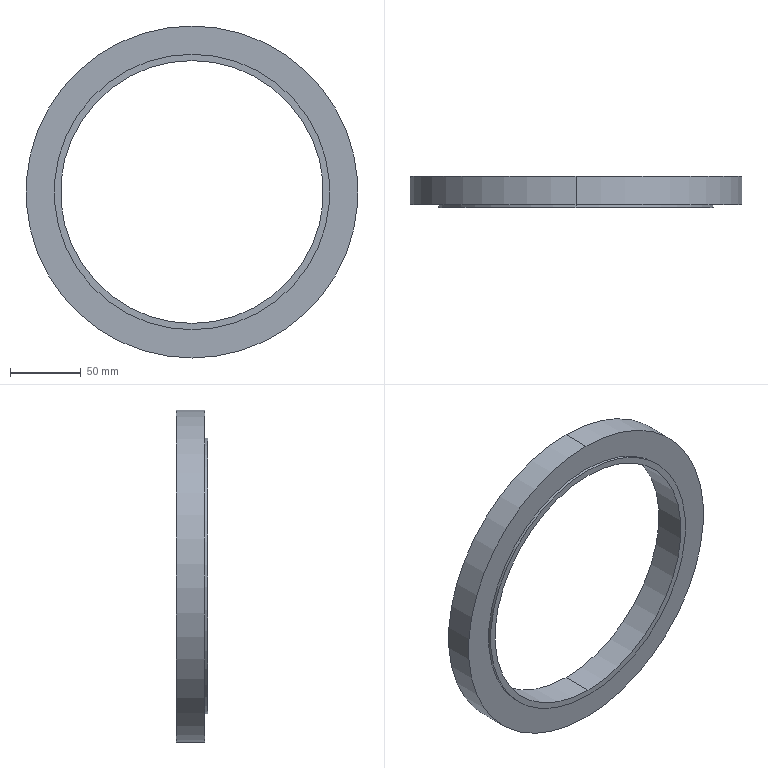Part | SolidWorks | features CirPattern 1, FlatPattern 1, HoleWzd 1, ICE 1, SMBaseFlange 1, SheetMetal 1 | 1 solid | 33 faces | box 235 x 22 x 235 mm | volume 321081 mm3 | cylinder 18 | cone 12 | plane 3 | commonest cylinder face diameters 10.2 x12 186 x2 195 x2 235 x2
STEP:
#1=CARTESIAN_POINT('',(90.933,-16.,-57.6));
#2=VERTEX_POINT('',#1);
#3=CARTESIAN_POINT('',(90.933,-16.,-47.4));
#4=VERTEX_POINT('',#3);
#5=CARTESIAN_POINT('',(90.933,-16.,-52.5));
#6=DIRECTION('',(0.,1.,0.));
#7=DIRECTION('',(0.,0.,1.));
#8=AXIS2_PLACEMENT_3D('',#5,#6,#7);
#9=CIRCLE('',#8,5.1);
#10=EDGE_CURVE('',#2,#4,#9,.T.);
#11=ORIENTED_EDGE('',*,*,#10,.F.);
#12=CARTESIAN_POINT('',(90.933,0.,-57.6));
#13=VERTEX_POINT('',#12);
#14=CARTESIAN_POINT('',(90.933,0.,-57.6));
#15=DIRECTION('',(0.,1.,0.));
#16=VECTOR('',#15,1000.);
#17=LINE('',#14,#16);
#18=EDGE_CURVE('',#2,#13,#17,.T.);
#19=ORIENTED_EDGE('',*,*,#18,.T.);
#20=CARTESIAN_POINT('',(90.933,0.,-47.4));
#21=VERTEX_POINT('',#20);
#22=CARTESIAN_POINT('',(90.933,0.,-52.5));
#23=DIRECTION('',(0.,1.,0.));
#24=DIRECTION('',(0.,0.,1.));
#25=AXIS2_PLACEMENT_3D('',#22,#23,#24);
#26=CIRCLE('',#25,5.1);
#27=EDGE_CURVE('',#13,#21,#26,.T.);
#28=ORIENTED_EDGE('',*,*,#27,.T.);
#29=CARTESIAN_POINT('',(90.933,0.,-47.4));
#30=DIRECTION('',(0.,1.,0.));
#31=VECTOR('',#30,1000.);
#32=LINE('',#29,#31);
#33=EDGE_CURVE('',#4,#21,#32,.T.);
#34=ORIENTED_EDGE('',*,*,#33,.F.);
#35=EDGE_LOOP('',(#11,#19,#28,#34));
#36=FACE_OUTER_BOUND('',#35,.T.);
#37=CARTESIAN_POINT('',(90.933,0.,-52.5));
#38=DIRECTION('',(0.,1.,0.));
#39=DIRECTION('',(0.,0.,1.));
#40=AXIS2_PLACEMENT_3D('',#37,#38,#39);
#41=CYLINDRICAL_SURFACE('',#40,5.1);
#42=ADVANCED_FACE('',(#36),#41,.F.);
#43=CARTESIAN_POINT('',(90.933,-19.064,-52.5));
#44=VERTEX_POINT('',#43);
#45=CARTESIAN_POINT('',(90.933,-16.,-47.4));
#46=DIRECTION('',(0.,0.515,0.8572));
#47=VECTOR('',#46,1000.);
#48=LINE('',#45,#47);
#49=EDGE_CURVE('',#44,#4,#48,.T.);
#50=ORIENTED_EDGE('',*,*,#49,.F.);
#51=CARTESIAN_POINT('',(90.933,-16.,-57.6));
#52=DIRECTION('',(0.,0.515,-0.8572));
#53=VECTOR('',#52,1000.);
#54=LINE('',#51,#53);
#55=EDGE_CURVE('',#44,#2,#54,.T.);
#56=ORIENTED_EDGE('',*,*,#55,.T.);
#57=ORIENTED_EDGE('',*,*,#10,.T.);
#58=EDGE_LOOP('',(#50,#56,#57));
#59=FACE_OUTER_BOUND('',#58,.T.);
#60=CARTESIAN_POINT('',(90.933,-16.,-52.5));
#61=DIRECTION('',(0.,1.,0.));
#62=DIRECTION('',(0.,0.,1.));
#63=AXIS2_PLACEMENT_3D('',#60,#61,#62);
#64=CONICAL_SURFACE('',#63,5.1,1.03);
#65=ADVANCED_FACE('',(#59),#64,.F.);
#66=CARTESIAN_POINT('',(90.933,-16.,47.4));
#67=VERTEX_POINT('',#66);
#68=CARTESIAN_POINT('',(90.933,-16.,57.6));
#69=VERTEX_POINT('',#68);
#70=CARTESIAN_POINT('',(90.933,-16.,52.5));
#71=DIRECTION('',(0.,1.,0.));
#72=DIRECTION('',(0.,0.,1.));
#73=AXIS2_PLACEMENT_3D('',#70,#71,#72);
#74=CIRCLE('',#73,5.1);
#75=EDGE_CURVE('',#67,#69,#74,.T.);
#76=ORIENTED_EDGE('',*,*,#75,.F.);
#77=CARTESIAN_POINT('',(90.933,0.,47.4));
#78=VERTEX_POINT('',#77);
#79=CARTESIAN_POINT('',(90.933,0.,47.4));
#80=DIRECTION('',(0.,1.,0.));
#81=VECTOR('',#80,1000.);
#82=LINE('',#79,#81);
#83=EDGE_CURVE('',#67,#78,#82,.T.);
#84=ORIENTED_EDGE('',*,*,#83,.T.);
#85=CARTESIAN_POINT('',(90.933,0.,57.6));
#86=VERTEX_POINT('',#85);
#87=CARTESIAN_POINT('',(90.933,0.,52.5));
#88=DIRECTION('',(0.,1.,0.));
#89=DIRECTION('',(0.,0.,1.));
#90=AXIS2_PLACEMENT_3D('',#87,#88,#89);
#91=CIRCLE('',#90,5.1);
#92=EDGE_CURVE('',#78,#86,#91,.T.);
#93=ORIENTED_EDGE('',*,*,#92,.T.);
#94=CARTESIAN_POINT('',(90.933,0.,57.6));
#95=DIRECTION('',(0.,1.,0.));
#96=VECTOR('',#95,1000.);
#97=LINE('',#94,#96);
#98=EDGE_CURVE('',#69,#86,#97,.T.);
#99=ORIENTED_EDGE('',*,*,#98,.F.);
#100=EDGE_LOOP('',(#76,#84,#93,#99));
#101=FACE_OUTER_BOUND('',#100,.T.);
#102=CARTESIAN_POINT('',(90.933,0.,52.5));
#103=DIRECTION('',(0.,1.,0.));
#104=DIRECTION('',(0.,0.,1.));
#105=AXIS2_PLACEMENT_3D('',#102,#103,#104);
#106=CYLINDRICAL_SURFACE('',#105,5.1);
#107=ADVANCED_FACE('',(#101),#106,.F.);
#108=CARTESIAN_POINT('',(90.933,-19.064,52.5));
#109=VERTEX_POINT('',#108);
#110=CARTESIAN_POINT('',(90.933,-16.,57.6));
#111=DIRECTION('',(0.,0.515,0.8572));
#112=VECTOR('',#111,1000.);
#113=LINE('',#110,#112);
#114=EDGE_CURVE('',#109,#69,#113,.T.);
#115=ORIENTED_EDGE('',*,*,#114,.F.);
#116=CARTESIAN_POINT('',(90.933,-16.,47.4));
#117=DIRECTION('',(0.,0.515,-0.8572));
#118=VECTOR('',#117,1000.);
#119=LINE('',#116,#118);
#120=EDGE_CURVE('',#109,#67,#119,.T.);
#121=ORIENTED_EDGE('',*,*,#120,.T.);
#122=ORIENTED_EDGE('',*,*,#75,.T.);
#123=EDGE_LOOP('',(#115,#121,#122));
#124=FACE_OUTER_BOUND('',#123,.T.);
#125=CARTESIAN_POINT('',(90.933,-16.,52.5));
#126=DIRECTION('',(0.,1.,0.));
#127=DIRECTION('',(0.,0.,1.));
#128=AXIS2_PLACEMENT_3D('',#125,#126,#127);
#129=CONICAL_SURFACE('',#128,5.1,1.03);
#130=ADVANCED_FACE('',(#124),#129,.F.);
#131=CARTESIAN_POINT('',(0.,-16.,99.9));
#132=VERTEX_POINT('',#131);
#133=CARTESIAN_POINT('',(0.,-16.,110.1));
#134=VERTEX_POINT('',#133);
#135=CARTESIAN_POINT('',(0.,-16.,105.));
#136=DIRECTION('',(0.,1.,0.));
#137=DIRECTION('',(0.,0.,1.));
#138=AXIS2_PLACEMENT_3D('',#135,#136,#137);
#139=CIRCLE('',#138,5.1);
#140=EDGE_CURVE('',#132,#134,#139,.T.);
#141=ORIENTED_EDGE('',*,*,#140,.F.);
#142=CARTESIAN_POINT('',(0.,0.,99.9));
#143=VERTEX_POINT('',#142);
#144=CARTESIAN_POINT('',(0.,0.,99.9));
#145=DIRECTION('',(0.,1.,0.));
#146=VECTOR('',#145,1000.);
#147=LINE('',#144,#146);
#148=EDGE_CURVE('',#132,#143,#147,.T.);
#149=ORIENTED_EDGE('',*,*,#148,.T.);
#150=CARTESIAN_POINT('',(0.,0.,110.1));
#151=VERTEX_POINT('',#150);
#152=CARTESIAN_POINT('',(0.,0.,105.));
#153=DIRECTION('',(0.,1.,0.));
#154=DIRECTION('',(0.,0.,1.));
#155=AXIS2_PLACEMENT_3D('',#152,#153,#154);
#156=CIRCLE('',#155,5.1);
#157=EDGE_CURVE('',#143,#151,#156,.T.);
#158=ORIENTED_EDGE('',*,*,#157,.T.);
#159=CARTESIAN_POINT('',(0.,0.,110.1));
#160=DIRECTION('',(0.,1.,0.));
#161=VECTOR('',#160,1000.);
#162=LINE('',#159,#161);
#163=EDGE_CURVE('',#134,#151,#162,.T.);
#164=ORIENTED_EDGE('',*,*,#163,.F.);
#165=EDGE_LOOP('',(#141,#149,#158,#164));
#166=FACE_OUTER_BOUND('',#165,.T.);
#167=CARTESIAN_POINT('',(0.,0.,105.));
#168=DIRECTION('',(0.,1.,0.));
#169=DIRECTION('',(0.,0.,1.));
#170=AXIS2_PLACEMENT_3D('',#167,#168,#169);
#171=CYLINDRICAL_SURFACE('',#170,5.1);
#172=ADVANCED_FACE('',(#166),#171,.F.);
#173=CARTESIAN_POINT('',(0.,-19.064,105.));
#174=VERTEX_POINT('',#173);
#175=CARTESIAN_POINT('',(0.,-16.,110.1));
#176=DIRECTION('',(0.,0.515,0.8572));
#177=VECTOR('',#176,1000.);
#178=LINE('',#175,#177);
#179=EDGE_CURVE('',#174,#134,#178,.T.);
#180=ORIENTED_EDGE('',*,*,#179,.F.);
#181=CARTESIAN_POINT('',(0.,-16.,99.9));
#182=DIRECTION('',(0.,0.515,-0.8572));
#183=VECTOR('',#182,1000.);
#184=LINE('',#181,#183);
#185=EDGE_CURVE('',#174,#132,#184,.T.);
#186=ORIENTED_EDGE('',*,*,#185,.T.);
#187=ORIENTED_EDGE('',*,*,#140,.T.);
#188=EDGE_LOOP('',(#180,#186,#187));
#189=FACE_OUTER_BOUND('',#188,.T.);
#190=CARTESIAN_POINT('',(0.,-16.,105.));
#191=DIRECTION('',(0.,1.,0.));
#192=DIRECTION('',(0.,0.,1.));
#193=AXIS2_PLACEMENT_3D('',#190,#191,#192);
#194=CONICAL_SURFACE('',#193,5.1,1.03);
#195=ADVANCED_FACE('',(#189),#194,.F.);
#196=CARTESIAN_POINT('',(-90.933,-16.,47.4));
#197=VERTEX_POINT('',#196);
#198=CARTESIAN_POINT('',(-90.933,-16.,57.6));
#199=VERTEX_POINT('',#198);
#200=CARTESIAN_POINT('',(-90.933,-16.,52.5));
#201=DIRECTION('',(0.,1.,0.));
#202=DIRECTION('',(0.,0.,1.));
#203=AXIS2_PLACEMENT_3D('',#200,#201,#202);
#204=CIRCLE('',#203,5.1);
#205=EDGE_CURVE('',#197,#199,#204,.T.);
#206=ORIENTED_EDGE('',*,*,#205,.F.);
#207=CARTESIAN_POINT('',(-90.933,0.,47.4));
#208=VERTEX_POINT('',#207);
#209=CARTESIAN_POINT('',(-90.933,0.,47.4));
#210=DIRECTION('',(0.,1.,0.));
#211=VECTOR('',#210,1000.);
#212=LINE('',#209,#211);
#213=EDGE_CURVE('',#197,#208,#212,.T.);
#214=ORIENTED_EDGE('',*,*,#213,.T.);
#215=CARTESIAN_POINT('',(-90.933,0.,57.6));
#216=VERTEX_POINT('',#215);
#217=CARTESIAN_POINT('',(-90.933,0.,52.5));
#218=DIRECTION('',(0.,1.,0.));
#219=DIRECTION('',(0.,0.,1.));
#220=AXIS2_PLACEMENT_3D('',#217,#218,#219);
#221=CIRCLE('',#220,5.1);
#222=EDGE_CURVE('',#208,#216,#221,.T.);
#223=ORIENTED_EDGE('',*,*,#222,.T.);
#224=CARTESIAN_POINT('',(-90.933,0.,57.6));
#225=DIRECTION('',(0.,1.,0.));
#226=VECTOR('',#225,1000.);
#227=LINE('',#224,#226);
#228=EDGE_CURVE('',#199,#216,#227,.T.);
#229=ORIENTED_EDGE('',*,*,#228,.F.);
#230=EDGE_LOOP('',(#206,#214,#223,#229));
#231=FACE_OUTER_BOUND('',#230,.T.);
#232=CARTESIAN_POINT('',(-90.933,0.,52.5));
#233=DIRECTION('',(0.,1.,0.));
#234=DIRECTION('',(0.,0.,1.));
#235=AXIS2_PLACEMENT_3D('',#232,#233,#234);
#236=CYLINDRICAL_SURFACE('',#235,5.1);
#237=ADVANCED_FACE('',(#231),#236,.F.);
#238=CARTESIAN_POINT('',(-90.933,-19.064,52.5));
#239=VERTEX_POINT('',#238);
#240=CARTESIAN_POINT('',(-90.933,-16.,57.6));
#241=DIRECTION('',(0.,0.515,0.8572));
#242=VECTOR('',#241,1000.);
#243=LINE('',#240,#242);
#244=EDGE_CURVE('',#239,#199,#243,.T.);
#245=ORIENTED_EDGE('',*,*,#244,.F.);
#246=CARTESIAN_POINT('',(-90.933,-16.,47.4));
#247=DIRECTION('',(0.,0.515,-0.8572));
#248=VECTOR('',#247,1000.);
#249=LINE('',#246,#248);
#250=EDGE_CURVE('',#239,#197,#249,.T.);
#251=ORIENTED_EDGE('',*,*,#250,.T.);
#252=ORIENTED_EDGE('',*,*,#205,.T.);
#253=EDGE_LOOP('',(#245,#251,#252));
#254=FACE_OUTER_BOUND('',#253,.T.);
#255=CARTESIAN_POINT('',(-90.933,-16.,52.5));
#256=DIRECTION('',(0.,1.,0.));
#257=DIRECTION('',(0.,0.,1.));
#258=AXIS2_PLACEMENT_3D('',#255,#256,#257);
#259=CONICAL_SURFACE('',#258,5.1,1.03);
#260=ADVANCED_FACE('',(#254),#259,.F.);
#261=CARTESIAN_POINT('',(-90.933,-16.,-57.6));
#262=VERTEX_POINT('',#261);
#263=CARTESIAN_POINT('',(-90.933,-16.,-47.4));
#264=VERTEX_POINT('',#263);
#265=CARTESIAN_POINT('',(-90.933,-16.,-52.5));
#266=DIRECTION('',(0.,1.,0.));
#267=DIRECTION('',(0.,0.,1.));
#268=AXIS2_PLACEMENT_3D('',#265,#266,#267);
#269=CIRCLE('',#268,5.1);
#270=EDGE_CURVE('',#262,#264,#269,.T.);
#271=ORIENTED_EDGE('',*,*,#270,.F.);
#272=CARTESIAN_POINT('',(-90.933,0.,-57.6));
#273=VERTEX_POINT('',#272);
#274=CARTESIAN_POINT('',(-90.933,0.,-57.6));
#275=DIRECTION('',(0.,1.,0.));
#276=VECTOR('',#275,1000.);
#277=LINE('',#274,#276);
#278=EDGE_CURVE('',#262,#273,#277,.T.);
#279=ORIENTED_EDGE('',*,*,#278,.T.);
#280=CARTESIAN_POINT('',(-90.933,0.,-47.4));
#281=VERTEX_POINT('',#280);
#282=CARTESIAN_POINT('',(-90.933,0.,-52.5));
#283=DIRECTION('',(0.,1.,0.));
#284=DIRECTION('',(0.,0.,1.));
#285=AXIS2_PLACEMENT_3D('',#282,#283,#284);
#286=CIRCLE('',#285,5.1);
#287=EDGE_CURVE('',#273,#281,#286,.T.);
#288=ORIENTED_EDGE('',*,*,#287,.T.);
#289=CARTESIAN_POINT('',(-90.933,0.,-47.4));
#290=DIRECTION('',(0.,1.,0.));
#291=VECTOR('',#290,1000.);
#292=LINE('',#289,#291);
#293=EDGE_CURVE('',#264,#281,#292,.T.);
#294=ORIENTED_EDGE('',*,*,#293,.F.);
#295=EDGE_LOOP('',(#271,#279,#288,#294));
#296=FACE_OUTER_BOUND('',#295,.T.);
#297=CARTESIAN_POINT('',(-90.933,0.,-52.5));
#298=DIRECTION('',(0.,1.,0.));
#299=DIRECTION('',(0.,0.,1.));
#300=AXIS2_PLACEMENT_3D('',#297,#298,#299);
#301=CYLINDRICAL_SURFACE('',#300,5.1);
#302=ADVANCED_FACE('',(#296),#301,.F.);
#303=CARTESIAN_POINT('',(-90.933,-19.064,-52.5));
#304=VERTEX_POINT('',#303);
#305=CARTESIAN_POINT('',(-90.933,-16.,-47.4));
#306=DIRECTION('',(0.,0.515,0.8572));
#307=VECTOR('',#306,1000.);
#308=LINE('',#305,#307);
#309=EDGE_CURVE('',#304,#264,#308,.T.);
#310=ORIENTED_EDGE('',*,*,#309,.F.);
#311=CARTESIAN_POINT('',(-90.933,-16.,-57.6));
#312=DIRECTION('',(0.,0.515,-0.8572));
#313=VECTOR('',#312,1000.);
#314=LINE('',#311,#313);
#315=EDGE_CURVE('',#304,#262,#314,.T.);
#316=ORIENTED_EDGE('',*,*,#315,.T.);
#317=ORIENTED_EDGE('',*,*,#270,.T.);
#318=EDGE_LOOP('',(#310,#316,#317));
#319=FACE_OUTER_BOUND('',#318,.T.);
#320=CARTESIAN_POINT('',(-90.933,-16.,-52.5));
#321=DIRECTION('',(0.,1.,0.));
#322=DIRECTION('',(0.,0.,1.));
#323=AXIS2_PLACEMENT_3D('',#320,#321,#322);
#324=CONICAL_SURFACE('',#323,5.1,1.03);
#325=ADVANCED_FACE('',(#319),#324,.F.);
#326=CARTESIAN_POINT('',(0.,-16.,-110.1));
#327=VERTEX_POINT('',#326);
#328=CARTESIAN_POINT('',(0.,-16.,-99.9));
#329=VERTEX_POINT('',#328);
#330=CARTESIAN_POINT('',(0.,-16.,-105.));
#331=DIRECTION('',(0.,1.,0.));
#332=DIRECTION('',(0.,0.,1.));
#333=AXIS2_PLACEMENT_3D('',#330,#331,#332);
#334=CIRCLE('',#333,5.1);
#335=EDGE_CURVE('',#327,#329,#334,.T.);
#336=ORIENTED_EDGE('',*,*,#335,.F.);
#337=CARTESIAN_POINT('',(0.,0.,-110.1));
#338=VERTEX_POINT('',#337);
#339=CARTESIAN_POINT('',(0.,0.,-110.1));
#340=DIRECTION('',(0.,1.,0.));
#341=VECTOR('',#340,1000.);
#342=LINE('',#339,#341);
#343=EDGE_CURVE('',#327,#338,#342,.T.);
#344=ORIENTED_EDGE('',*,*,#343,.T.);
#345=CARTESIAN_POINT('',(0.,0.,-99.9));
#346=VERTEX_POINT('',#345);
#347=CARTESIAN_POINT('',(0.,0.,-105.));
#348=DIRECTION('',(0.,1.,0.));
#349=DIRECTION('',(0.,0.,1.));
#350=AXIS2_PLACEMENT_3D('',#347,#348,#349);
#351=CIRCLE('',#350,5.1);
#352=EDGE_CURVE('',#338,#346,#351,.T.);
#353=ORIENTED_EDGE('',*,*,#352,.T.);
#354=CARTESIAN_POINT('',(0.,0.,-99.9));
#355=DIRECTION('',(0.,1.,0.));
#356=VECTOR('',#355,1000.);
#357=LINE('',#354,#356);
#358=EDGE_CURVE('',#329,#346,#357,.T.);
#359=ORIENTED_EDGE('',*,*,#358,.F.);
#360=EDGE_LOOP('',(#336,#344,#353,#359));
#361=FACE_OUTER_BOUND('',#360,.T.);
#362=CARTESIAN_POINT('',(0.,0.,-105.));
#363=DIRECTION('',(0.,1.,0.));
#364=DIRECTION('',(0.,0.,1.));
#365=AXIS2_PLACEMENT_3D('',#362,#363,#364);
#366=CYLINDRICAL_SURFACE('',#365,5.1);
#367=ADVANCED_FACE('',(#361),#366,.F.);
#368=CARTESIAN_POINT('',(0.,-19.064,-105.));
#369=VERTEX_POINT('',#368);
#370=CARTESIAN_POINT('',(0.,-16.,-99.9));
#371=DIRECTION('',(0.,0.515,0.8572));
#372=VECTOR('',#371,1000.);
#373=LINE('',#370,#372);
#374=EDGE_CURVE('',#369,#329,#373,.T.);
#375=ORIENTED_EDGE('',*,*,#374,.F.);
#376=CARTESIAN_POINT('',(0.,-16.,-110.1));
#377=DIRECTION('',(0.,0.515,-0.8572));
#378=VECTOR('',#377,1000.);
#379=LINE('',#376,#378);
#380=EDGE_CURVE('',#369,#327,#379,.T.);
#381=ORIENTED_EDGE('',*,*,#380,.T.);
#382=ORIENTED_EDGE('',*,*,#335,.T.);
#383=EDGE_LOOP('',(#375,#381,#382));
#384=FACE_OUTER_BOUND('',#383,.T.);
#385=CARTESIAN_POINT('',(0.,-16.,-105.));
#386=DIRECTION('',(0.,1.,0.));
#387=DIRECTION('',(0.,0.,1.));
#388=AXIS2_PLACEMENT_3D('',#385,#386,#387);
#389=CONICAL_SURFACE('',#388,5.1,1.03);
#390=ADVANCED_FACE('',(#384),#389,.F.);
#391=CARTESIAN_POINT('',(0.,-20.,-97.5));
#392=VERTEX_POINT('',#391);
#393=CARTESIAN_POINT('',(0.,-20.,97.5));
#394=VERTEX_POINT('',#393);
#395=CARTESIAN_POINT('',(0.,-20.,0.));
#396=DIRECTION('',(0.,-1.,0.));
#397=DIRECTION('',(0.,0.,-1.));
#398=AXIS2_PLACEMENT_3D('',#395,#396,#397);
#399=CIRCLE('',#398,97.5);
#400=EDGE_CURVE('',#392,#394,#399,.T.);
#401=ORIENTED_EDGE('',*,*,#400,.T.);
#402=CARTESIAN_POINT('',(0.,-22.,97.5));
#403=VERTEX_POINT('',#402);
#404=CARTESIAN_POINT('',(0.,-20.,97.5));
#405=DIRECTION('',(0.,-1.,0.));
#406=VECTOR('',#405,1000.);
#407=LINE('',#404,#406);
#408=EDGE_CURVE('',#394,#403,#407,.T.);
#409=ORIENTED_EDGE('',*,*,#408,.T.);
#410=CARTESIAN_POINT('',(0.,-22.,-97.5));
#411=VERTEX_POINT('',#410);
#412=CARTESIAN_POINT('',(0.,-22.,0.));
#413=DIRECTION('',(0.,-1.,0.));
#414=DIRECTION('',(0.,0.,-1.));
#415=AXIS2_PLACEMENT_3D('',#412,#413,#414);
#416=CIRCLE('',#415,97.5);
#417=EDGE_CURVE('',#411,#403,#416,.T.);
#418=ORIENTED_EDGE('',*,*,#417,.F.);
#419=CARTESIAN_POINT('',(0.,-20.,-97.5));
#420=DIRECTION('',(0.,-1.,0.));
#421=VECTOR('',#420,1000.);
#422=LINE('',#419,#421);
#423=EDGE_CURVE('',#392,#411,#422,.T.);
#424=ORIENTED_EDGE('',*,*,#423,.F.);
#425=EDGE_LOOP('',(#401,#409,#418,#424));
#426=FACE_OUTER_BOUND('',#425,.T.);
#427=CARTESIAN_POINT('',(0.,-20.,0.));
#428=DIRECTION('',(0.,-1.,0.));
#429=DIRECTION('',(0.,0.,-1.));
#430=AXIS2_PLACEMENT_3D('',#427,#428,#429);
#431=CYLINDRICAL_SURFACE('',#430,97.5);
#432=ADVANCED_FACE('',(#426),#431,.T.);
#433=CARTESIAN_POINT('',(0.,-22.,-93.));
#434=VERTEX_POINT('',#433);
#435=CARTESIAN_POINT('',(0.,-22.,93.));
#436=VERTEX_POINT('',#435);
#437=CARTESIAN_POINT('',(0.,-22.,0.));
#438=DIRECTION('',(0.,1.,0.));
#439=DIRECTION('',(0.,0.,1.));
#440=AXIS2_PLACEMENT_3D('',#437,#438,#439);
#441=CIRCLE('',#440,93.);
#442=EDGE_CURVE('',#434,#436,#441,.T.);
#443=ORIENTED_EDGE('',*,*,#442,.F.);
#444=CARTESIAN_POINT('',(0.,0.,-93.));
#445=VERTEX_POINT('',#444);
#446=CARTESIAN_POINT('',(0.,-22.,-93.));
#447=DIRECTION('',(0.,1.,0.));
#448=VECTOR('',#447,1000.);
#449=LINE('',#446,#448);
#450=EDGE_CURVE('',#434,#445,#449,.T.);
#451=ORIENTED_EDGE('',*,*,#450,.T.);
#452=CARTESIAN_POINT('',(0.,0.,93.));
#453=VERTEX_POINT('',#452);
#454=CARTESIAN_POINT('',(0.,0.,0.));
#455=DIRECTION('',(0.,1.,0.));
#456=DIRECTION('',(0.,0.,1.));
#457=AXIS2_PLACEMENT_3D('',#454,#455,#456);
#458=CIRCLE('',#457,93.);
#459=EDGE_CURVE('',#445,#453,#458,.T.);
#460=ORIENTED_EDGE('',*,*,#459,.T.);
#461=CARTESIAN_POINT('',(0.,-22.,93.));
#462=DIRECTION('',(0.,1.,0.));
#463=VECTOR('',#462,1000.);
#464=LINE('',#461,#463);
#465=EDGE_CURVE('',#436,#453,#464,.T.);
#466=ORIENTED_EDGE('',*,*,#465,.F.);
#467=EDGE_LOOP('',(#443,#451,#460,#466));
#468=FACE_OUTER_BOUND('',#467,.T.);
#469=CARTESIAN_POINT('',(0.,-22.,0.));
#470=DIRECTION('',(0.,1.,0.));
#471=DIRECTION('',(0.,0.,1.));
#472=AXIS2_PLACEMENT_3D('',#469,#470,#471);
#473=CYLINDRICAL_SURFACE('',#472,93.);
#474=ADVANCED_FACE('',(#468),#473,.F.);
#475=CARTESIAN_POINT('',(0.,-20.,117.5));
#476=VERTEX_POINT('',#475);
#477=CARTESIAN_POINT('',(0.,-20.,-117.5));
#478=VERTEX_POINT('',#477);
#479=CARTESIAN_POINT('',(0.,-20.,0.));
#480=DIRECTION('',(0.,1.,0.));
#481=DIRECTION('',(0.,0.,-1.));
#482=AXIS2_PLACEMENT_3D('',#479,#480,#481);
#483=CIRCLE('',#482,117.5);
#484=EDGE_CURVE('',#476,#478,#483,.T.);
#485=ORIENTED_EDGE('',*,*,#484,.T.);
#486=CARTESIAN_POINT('',(0.,0.,-117.5));
#487=VERTEX_POINT('',#486);
#488=CARTESIAN_POINT('',(0.,-22.,-117.5));
#489=DIRECTION('',(0.,1.,0.));
#490=VECTOR('',#489,1000.);
#491=LINE('',#488,#490);
#492=EDGE_CURVE('',#478,#487,#491,.T.);
#493=ORIENTED_EDGE('',*,*,#492,.T.);
#494=CARTESIAN_POINT('',(0.,0.,117.5));
#495=VERTEX_POINT('',#494);
#496=CARTESIAN_POINT('',(0.,0.,0.));
#497=DIRECTION('',(0.,1.,0.));
#498=DIRECTION('',(0.,0.,1.));
#499=AXIS2_PLACEMENT_3D('',#496,#497,#498);
#500=CIRCLE('',#499,117.5);
#501=EDGE_CURVE('',#495,#487,#500,.T.);
#502=ORIENTED_EDGE('',*,*,#501,.F.);
#503=CARTESIAN_POINT('',(0.,-22.,117.5));
#504=DIRECTION('',(0.,1.,0.));
#505=VECTOR('',#504,1000.);
#506=LINE('',#503,#505);
#507=EDGE_CURVE('',#476,#495,#506,.T.);
#508=ORIENTED_EDGE('',*,*,#507,.F.);
#509=EDGE_LOOP('',(#485,#493,#502,#508));
#510=FACE_OUTER_BOUND('',#509,.T.);
#511=CARTESIAN_POINT('',(0.,-22.,0.));
#512=DIRECTION('',(0.,1.,0.));
#513=DIRECTION('',(0.,0.,1.));
#514=AXIS2_PLACEMENT_3D('',#511,#512,#513);
#515=CYLINDRICAL_SURFACE('',#514,117.5);
#516=ADVANCED_FACE('',(#510),#515,.T.);
#517=ORIENTED_EDGE('',*,*,#492,.F.);
#518=CARTESIAN_POINT('',(0.,-20.,0.));
#519=DIRECTION('',(0.,1.,0.));
#520=DIRECTION('',(0.,0.,-1.));
#521=AXIS2_PLACEMENT_3D('',#518,#519,#520);
#522=CIRCLE('',#521,117.5);
#523=EDGE_CURVE('',#478,#476,#522,.T.);
#524=ORIENTED_EDGE('',*,*,#523,.T.);
#525=ORIENTED_EDGE('',*,*,#507,.T.);
#526=CARTESIAN_POINT('',(0.,0.,0.));
#527=DIRECTION('',(0.,1.,0.));
#528=DIRECTION('',(0.,0.,1.));
#529=AXIS2_PLACEMENT_3D('',#526,#527,#528);
#530=CIRCLE('',#529,117.5);
#531=EDGE_CURVE('',#487,#495,#530,.T.);
#532=ORIENTED_EDGE('',*,*,#531,.F.);
#533=EDGE_LOOP('',(#517,#524,#525,#532));
#534=FACE_OUTER_BOUND('',#533,.T.);
#535=CARTESIAN_POINT('',(0.,-22.,0.));
#536=DIRECTION('',(0.,1.,0.));
#537=DIRECTION('',(0.,0.,1.));
#538=AXIS2_PLACEMENT_3D('',#535,#536,#537);
#539=CYLINDRICAL_SURFACE('',#538,117.5);
#540=ADVANCED_FACE('',(#534),#539,.T.);
#541=CARTESIAN_POINT('',(0.,-22.,0.));
#542=DIRECTION('',(0.,1.,0.));
#543=DIRECTION('',(0.,0.,1.));
#544=AXIS2_PLACEMENT_3D('',#541,#542,#543);
#545=CIRCLE('',#544,93.);
#546=EDGE_CURVE('',#436,#434,#545,.T.);
#547=ORIENTED_EDGE('',*,*,#546,.T.);
#548=ORIENTED_EDGE('',*,*,#442,.T.);
#549=EDGE_LOOP('',(#547,#548));
#550=FACE_BOUND('',#549,.T.);
#551=ORIENTED_EDGE('',*,*,#417,.T.);
#552=CARTESIAN_POINT('',(0.,-22.,0.));
#553=DIRECTION('',(0.,-1.,0.));
#554=DIRECTION('',(0.,0.,-1.));
#555=AXIS2_PLACEMENT_3D('',#552,#553,#554);
#556=CIRCLE('',#555,97.5);
#557=EDGE_CURVE('',#403,#411,#556,.T.);
#558=ORIENTED_EDGE('',*,*,#557,.T.);
#559=EDGE_LOOP('',(#551,#558));
#560=FACE_OUTER_BOUND('',#559,.T.);
#561=CARTESIAN_POINT('',(0.,-22.,0.));
#562=DIRECTION('',(0.,1.,0.));
#563=DIRECTION('',(0.,0.,1.));
#564=AXIS2_PLACEMENT_3D('',#561,#562,#563);
#565=PLANE('',#564);
#566=ADVANCED_FACE('',(#550,#560),#565,.F.);
#567=CARTESIAN_POINT('',(90.933,0.,-52.5));
#568=DIRECTION('',(0.,1.,0.));
#569=DIRECTION('',(0.,0.,1.));
#570=AXIS2_PLACEMENT_3D('',#567,#568,#569);
#571=CIRCLE('',#570,5.1);
#572=EDGE_CURVE('',#21,#13,#571,.T.);
#573=ORIENTED_EDGE('',*,*,#572,.F.);
#574=ORIENTED_EDGE('',*,*,#27,.F.);
#575=EDGE_LOOP('',(#573,#574));
#576=FACE_BOUND('',#575,.T.);
#577=CARTESIAN_POINT('',(90.933,0.,52.5));
#578=DIRECTION('',(0.,1.,0.));
#579=DIRECTION('',(0.,0.,1.));
#580=AXIS2_PLACEMENT_3D('',#577,#578,#579);
#581=CIRCLE('',#580,5.1);
#582=EDGE_CURVE('',#86,#78,#581,.T.);
#583=ORIENTED_EDGE('',*,*,#582,.F.);
#584=ORIENTED_EDGE('',*,*,#92,.F.);
#585=EDGE_LOOP('',(#583,#584));
#586=FACE_BOUND('',#585,.T.);
#587=CARTESIAN_POINT('',(0.,0.,105.));
#588=DIRECTION('',(0.,1.,0.));
#589=DIRECTION('',(0.,0.,1.));
#590=AXIS2_PLACEMENT_3D('',#587,#588,#589);
#591=CIRCLE('',#590,5.1);
#592=EDGE_CURVE('',#151,#143,#591,.T.);
#593=ORIENTED_EDGE('',*,*,#592,.F.);
#594=ORIENTED_EDGE('',*,*,#157,.F.);
#595=EDGE_LOOP('',(#593,#594));
#596=FACE_BOUND('',#595,.T.);
#597=CARTESIAN_POINT('',(-90.933,0.,52.5));
#598=DIRECTION('',(0.,1.,0.));
#599=DIRECTION('',(0.,0.,1.));
#600=AXIS2_PLACEMENT_3D('',#597,#598,#599);
#601=CIRCLE('',#600,5.1);
#602=EDGE_CURVE('',#216,#208,#601,.T.);
#603=ORIENTED_EDGE('',*,*,#602,.F.);
#604=ORIENTED_EDGE('',*,*,#222,.F.);
#605=EDGE_LOOP('',(#603,#604));
#606=FACE_BOUND('',#605,.T.);
#607=CARTESIAN_POINT('',(-90.933,0.,-52.5));
#608=DIRECTION('',(0.,1.,0.));
#609=DIRECTION('',(0.,0.,1.));
#610=AXIS2_PLACEMENT_3D('',#607,#608,#609);
#611=CIRCLE('',#610,5.1);
#612=EDGE_CURVE('',#281,#273,#611,.T.);
#613=ORIENTED_EDGE('',*,*,#612,.F.);
#614=ORIENTED_EDGE('',*,*,#287,.F.);
#615=EDGE_LOOP('',(#613,#614));
#616=FACE_BOUND('',#615,.T.);
#617=CARTESIAN_POINT('',(0.,0.,-105.));
#618=DIRECTION('',(0.,1.,0.));
#619=DIRECTION('',(0.,0.,1.));
#620=AXIS2_PLACEMENT_3D('',#617,#618,#619);
#621=CIRCLE('',#620,5.1);
#622=EDGE_CURVE('',#346,#338,#621,.T.);
#623=ORIENTED_EDGE('',*,*,#622,.F.);
#624=ORIENTED_EDGE('',*,*,#352,.F.);
#625=EDGE_LOOP('',(#623,#624));
#626=FACE_BOUND('',#625,.T.);
#627=CARTESIAN_POINT('',(0.,0.,0.));
#628=DIRECTION('',(0.,1.,0.));
#629=DIRECTION('',(0.,0.,1.));
#630=AXIS2_PLACEMENT_3D('',#627,#628,#629);
#631=CIRCLE('',#630,93.);
#632=EDGE_CURVE('',#453,#445,#631,.T.);
#633=ORIENTED_EDGE('',*,*,#632,.F.);
#634=ORIENTED_EDGE('',*,*,#459,.F.);
#635=EDGE_LOOP('',(#633,#634));
#636=FACE_BOUND('',#635,.T.);
#637=ORIENTED_EDGE('',*,*,#501,.T.);
#638=ORIENTED_EDGE('',*,*,#531,.T.);
#639=EDGE_LOOP('',(#637,#638));
#640=FACE_OUTER_BOUND('',#639,.T.);
#641=CARTESIAN_POINT('',(0.,0.,0.));
#642=DIRECTION('',(0.,1.,0.));
#643=DIRECTION('',(0.,0.,1.));
#644=AXIS2_PLACEMENT_3D('',#641,#642,#643);
#645=PLANE('',#644);
#646=ADVANCED_FACE('',(#576,#586,#596,#606,#616,#626,#636,#640),#645,.T.);
#647=ORIENTED_EDGE('',*,*,#450,.F.);
#648=ORIENTED_EDGE('',*,*,#546,.F.);
#649=ORIENTED_EDGE('',*,*,#465,.T.);
#650=ORIENTED_EDGE('',*,*,#632,.T.);
#651=EDGE_LOOP('',(#647,#648,#649,#650));
#652=FACE_OUTER_BOUND('',#651,.T.);
#653=CARTESIAN_POINT('',(0.,-22.,0.));
#654=DIRECTION('',(0.,1.,0.));
#655=DIRECTION('',(0.,0.,1.));
#656=AXIS2_PLACEMENT_3D('',#653,#654,#655);
#657=CYLINDRICAL_SURFACE('',#656,93.);
#658=ADVANCED_FACE('',(#652),#657,.F.);
#659=ORIENTED_EDGE('',*,*,#484,.F.);
#660=ORIENTED_EDGE('',*,*,#523,.F.);
#661=EDGE_LOOP('',(#659,#660));
#662=FACE_OUTER_BOUND('',#661,.T.);
#663=ORIENTED_EDGE('',*,*,#400,.F.);
#664=CARTESIAN_POINT('',(0.,-20.,0.));
#665=DIRECTION('',(0.,-1.,0.));
#666=DIRECTION('',(0.,0.,-1.));
#667=AXIS2_PLACEMENT_3D('',#664,#665,#666);
#668=CIRCLE('',#667,97.5);
#669=EDGE_CURVE('',#394,#392,#668,.T.);
#670=ORIENTED_EDGE('',*,*,#669,.F.);
#671=EDGE_LOOP('',(#663,#670));
#672=FACE_BOUND('',#671,.T.);
#673=CARTESIAN_POINT('',(0.,-20.,0.));
#674=DIRECTION('',(0.,-1.,0.));
#675=DIRECTION('',(0.,0.,-1.));
#676=AXIS2_PLACEMENT_3D('',#673,#674,#675);
#677=PLANE('',#676);
#678=ADVANCED_FACE('',(#662,#672),#677,.T.);
#679=ORIENTED_EDGE('',*,*,#408,.F.);
#680=ORIENTED_EDGE('',*,*,#669,.T.);
#681=ORIENTED_EDGE('',*,*,#423,.T.);
#682=ORIENTED_EDGE('',*,*,#557,.F.);
#683=EDGE_LOOP('',(#679,#680,#681,#682));
#684=FACE_OUTER_BOUND('',#683,.T.);
#685=CARTESIAN_POINT('',(0.,-20.,0.));
#686=DIRECTION('',(0.,-1.,0.));
#687=DIRECTION('',(0.,0.,-1.));
#688=AXIS2_PLACEMENT_3D('',#685,#686,#687);
#689=CYLINDRICAL_SURFACE('',#688,97.5);
#690=ADVANCED_FACE('',(#684),#689,.T.);
#691=ORIENTED_EDGE('',*,*,#380,.F.);
#692=ORIENTED_EDGE('',*,*,#374,.T.);
#693=CARTESIAN_POINT('',(0.,-16.,-105.));
#694=DIRECTION('',(0.,1.,0.));
#695=DIRECTION('',(0.,0.,1.));
#696=AXIS2_PLACEMENT_3D('',#693,#694,#695);
#697=CIRCLE('',#696,5.1);
#698=EDGE_CURVE('',#329,#327,#697,.T.);
#699=ORIENTED_EDGE('',*,*,#698,.T.);
#700=EDGE_LOOP('',(#691,#692,#699));
#701=FACE_OUTER_BOUND('',#700,.T.);
#702=CARTESIAN_POINT('',(0.,-16.,-105.));
#703=DIRECTION('',(0.,1.,0.));
#704=DIRECTION('',(0.,0.,1.));
#705=AXIS2_PLACEMENT_3D('',#702,#703,#704);
#706=CONICAL_SURFACE('',#705,5.1,1.03);
#707=ADVANCED_FACE('',(#701),#706,.F.);
#708=ORIENTED_EDGE('',*,*,#343,.F.);
#709=ORIENTED_EDGE('',*,*,#698,.F.);
#710=ORIENTED_EDGE('',*,*,#358,.T.);
#711=ORIENTED_EDGE('',*,*,#622,.T.);
#712=EDGE_LOOP('',(#708,#709,#710,#711));
#713=FACE_OUTER_BOUND('',#712,.T.);
#714=CARTESIAN_POINT('',(0.,0.,-105.));
#715=DIRECTION('',(0.,1.,0.));
#716=DIRECTION('',(0.,0.,1.));
#717=AXIS2_PLACEMENT_3D('',#714,#715,#716);
#718=CYLINDRICAL_SURFACE('',#717,5.1);
#719=ADVANCED_FACE('',(#713),#718,.F.);
#720=ORIENTED_EDGE('',*,*,#315,.F.);
#721=ORIENTED_EDGE('',*,*,#309,.T.);
#722=CARTESIAN_POINT('',(-90.933,-16.,-52.5));
#723=DIRECTION('',(0.,1.,0.));
#724=DIRECTION('',(0.,0.,1.));
#725=AXIS2_PLACEMENT_3D('',#722,#723,#724);
#726=CIRCLE('',#725,5.1);
#727=EDGE_CURVE('',#264,#262,#726,.T.);
#728=ORIENTED_EDGE('',*,*,#727,.T.);
#729=EDGE_LOOP('',(#720,#721,#728));
#730=FACE_OUTER_BOUND('',#729,.T.);
#731=CARTESIAN_POINT('',(-90.933,-16.,-52.5));
#732=DIRECTION('',(0.,1.,0.));
#733=DIRECTION('',(0.,0.,1.));
#734=AXIS2_PLACEMENT_3D('',#731,#732,#733);
#735=CONICAL_SURFACE('',#734,5.1,1.03);
#736=ADVANCED_FACE('',(#730),#735,.F.);
#737=ORIENTED_EDGE('',*,*,#278,.F.);
#738=ORIENTED_EDGE('',*,*,#727,.F.);
#739=ORIENTED_EDGE('',*,*,#293,.T.);
#740=ORIENTED_EDGE('',*,*,#612,.T.);
#741=EDGE_LOOP('',(#737,#738,#739,#740));
#742=FACE_OUTER_BOUND('',#741,.T.);
#743=CARTESIAN_POINT('',(-90.933,0.,-52.5));
#744=DIRECTION('',(0.,1.,0.));
#745=DIRECTION('',(0.,0.,1.));
#746=AXIS2_PLACEMENT_3D('',#743,#744,#745);
#747=CYLINDRICAL_SURFACE('',#746,5.1);
#748=ADVANCED_FACE('',(#742),#747,.F.);
#749=ORIENTED_EDGE('',*,*,#250,.F.);
#750=ORIENTED_EDGE('',*,*,#244,.T.);
#751=CARTESIAN_POINT('',(-90.933,-16.,52.5));
#752=DIRECTION('',(0.,1.,0.));
#753=DIRECTION('',(0.,0.,1.));
#754=AXIS2_PLACEMENT_3D('',#751,#752,#753);
#755=CIRCLE('',#754,5.1);
#756=EDGE_CURVE('',#199,#197,#755,.T.);
#757=ORIENTED_EDGE('',*,*,#756,.T.);
#758=EDGE_LOOP('',(#749,#750,#757));
#759=FACE_OUTER_BOUND('',#758,.T.);
#760=CARTESIAN_POINT('',(-90.933,-16.,52.5));
#761=DIRECTION('',(0.,1.,0.));
#762=DIRECTION('',(0.,0.,1.));
#763=AXIS2_PLACEMENT_3D('',#760,#761,#762);
#764=CONICAL_SURFACE('',#763,5.1,1.03);
#765=ADVANCED_FACE('',(#759),#764,.F.);
#766=ORIENTED_EDGE('',*,*,#213,.F.);
#767=ORIENTED_EDGE('',*,*,#756,.F.);
#768=ORIENTED_EDGE('',*,*,#228,.T.);
#769=ORIENTED_EDGE('',*,*,#602,.T.);
#770=EDGE_LOOP('',(#766,#767,#768,#769));
#771=FACE_OUTER_BOUND('',#770,.T.);
#772=CARTESIAN_POINT('',(-90.933,0.,52.5));
#773=DIRECTION('',(0.,1.,0.));
#774=DIRECTION('',(0.,0.,1.));
#775=AXIS2_PLACEMENT_3D('',#772,#773,#774);
#776=CYLINDRICAL_SURFACE('',#775,5.1);
#777=ADVANCED_FACE('',(#771),#776,.F.);
#778=ORIENTED_EDGE('',*,*,#185,.F.);
#779=ORIENTED_EDGE('',*,*,#179,.T.);
#780=CARTESIAN_POINT('',(0.,-16.,105.));
#781=DIRECTION('',(0.,1.,0.));
#782=DIRECTION('',(0.,0.,1.));
#783=AXIS2_PLACEMENT_3D('',#780,#781,#782);
#784=CIRCLE('',#783,5.1);
#785=EDGE_CURVE('',#134,#132,#784,.T.);
#786=ORIENTED_EDGE('',*,*,#785,.T.);
#787=EDGE_LOOP('',(#778,#779,#786));
#788=FACE_OUTER_BOUND('',#787,.T.);
#789=CARTESIAN_POINT('',(0.,-16.,105.));
#790=DIRECTION('',(0.,1.,0.));
#791=DIRECTION('',(0.,0.,1.));
#792=AXIS2_PLACEMENT_3D('',#789,#790,#791);
#793=CONICAL_SURFACE('',#792,5.1,1.03);
#794=ADVANCED_FACE('',(#788),#793,.F.);
#795=ORIENTED_EDGE('',*,*,#148,.F.);
#796=ORIENTED_EDGE('',*,*,#785,.F.);
#797=ORIENTED_EDGE('',*,*,#163,.T.);
#798=ORIENTED_EDGE('',*,*,#592,.T.);
#799=EDGE_LOOP('',(#795,#796,#797,#798));
#800=FACE_OUTER_BOUND('',#799,.T.);
#801=CARTESIAN_POINT('',(0.,0.,105.));
#802=DIRECTION('',(0.,1.,0.));
#803=DIRECTION('',(0.,0.,1.));
#804=AXIS2_PLACEMENT_3D('',#801,#802,#803);
#805=CYLINDRICAL_SURFACE('',#804,5.1);
#806=ADVANCED_FACE('',(#800),#805,.F.);
#807=ORIENTED_EDGE('',*,*,#120,.F.);
#808=ORIENTED_EDGE('',*,*,#114,.T.);
#809=CARTESIAN_POINT('',(90.933,-16.,52.5));
#810=DIRECTION('',(0.,1.,0.));
#811=DIRECTION('',(0.,0.,1.));
#812=AXIS2_PLACEMENT_3D('',#809,#810,#811);
#813=CIRCLE('',#812,5.1);
#814=EDGE_CURVE('',#69,#67,#813,.T.);
#815=ORIENTED_EDGE('',*,*,#814,.T.);
#816=EDGE_LOOP('',(#807,#808,#815));
#817=FACE_OUTER_BOUND('',#816,.T.);
#818=CARTESIAN_POINT('',(90.933,-16.,52.5));
#819=DIRECTION('',(0.,1.,0.));
#820=DIRECTION('',(0.,0.,1.));
#821=AXIS2_PLACEMENT_3D('',#818,#819,#820);
#822=CONICAL_SURFACE('',#821,5.1,1.03);
#823=ADVANCED_FACE('',(#817),#822,.F.);
#824=ORIENTED_EDGE('',*,*,#83,.F.);
#825=ORIENTED_EDGE('',*,*,#814,.F.);
#826=ORIENTED_EDGE('',*,*,#98,.T.);
#827=ORIENTED_EDGE('',*,*,#582,.T.);
#828=EDGE_LOOP('',(#824,#825,#826,#827));
#829=FACE_OUTER_BOUND('',#828,.T.);
#830=CARTESIAN_POINT('',(90.933,0.,52.5));
#831=DIRECTION('',(0.,1.,0.));
#832=DIRECTION('',(0.,0.,1.));
#833=AXIS2_PLACEMENT_3D('',#830,#831,#832);
#834=CYLINDRICAL_SURFACE('',#833,5.1);
#835=ADVANCED_FACE('',(#829),#834,.F.);
#836=ORIENTED_EDGE('',*,*,#55,.F.);
#837=ORIENTED_EDGE('',*,*,#49,.T.);
#838=CARTESIAN_POINT('',(90.933,-16.,-52.5));
#839=DIRECTION('',(0.,1.,0.));
#840=DIRECTION('',(0.,0.,1.));
#841=AXIS2_PLACEMENT_3D('',#838,#839,#840);
#842=CIRCLE('',#841,5.1);
#843=EDGE_CURVE('',#4,#2,#842,.T.);
#844=ORIENTED_EDGE('',*,*,#843,.T.);
#845=EDGE_LOOP('',(#836,#837,#844));
#846=FACE_OUTER_BOUND('',#845,.T.);
#847=CARTESIAN_POINT('',(90.933,-16.,-52.5));
#848=DIRECTION('',(0.,1.,0.));
#849=DIRECTION('',(0.,0.,1.));
#850=AXIS2_PLACEMENT_3D('',#847,#848,#849);
#851=CONICAL_SURFACE('',#850,5.1,1.03);
#852=ADVANCED_FACE('',(#846),#851,.F.);
#853=ORIENTED_EDGE('',*,*,#18,.F.);
#854=ORIENTED_EDGE('',*,*,#843,.F.);
#855=ORIENTED_EDGE('',*,*,#33,.T.);
#856=ORIENTED_EDGE('',*,*,#572,.T.);
#857=EDGE_LOOP('',(#853,#854,#855,#856));
#858=FACE_OUTER_BOUND('',#857,.T.);
#859=CARTESIAN_POINT('',(90.933,0.,-52.5));
#860=DIRECTION('',(0.,1.,0.));
#861=DIRECTION('',(0.,0.,1.));
#862=AXIS2_PLACEMENT_3D('',#859,#860,#861);
#863=CYLINDRICAL_SURFACE('',#862,5.1);
#864=ADVANCED_FACE('',(#858),#863,.F.);
#865=CLOSED_SHELL('',(#42,#65,#107,#130,#172,#195,#237,#260,#302,#325,#367,#390,#432,#474,#516,#540,#566,#646,#658,#678,#690,#707,#719,#736,#748,#765,#777,#794,#806,#823,#835,#852,#864));
#866=MANIFOLD_SOLID_BREP('',#865);
#867=CARTESIAN_POINT('',(0.,0.,0.));
#868=DIRECTION('',(0.,0.,1.));
#869=DIRECTION('',(1.,0.,0.));
#870=AXIS2_PLACEMENT_3D('',#867,#868,#869);
#871=(LENGTH_UNIT()NAMED_UNIT(*)SI_UNIT(.MILLI.,.METRE.));
#872=UNCERTAINTY_MEASURE_WITH_UNIT(LENGTH_MEASURE(0.00001),#871,'','');
#873=(NAMED_UNIT(*)PLANE_ANGLE_UNIT()SI_UNIT($,.RADIAN.));
#874=(NAMED_UNIT(*)SI_UNIT($,.STERADIAN.)SOLID_ANGLE_UNIT());
#875=(GEOMETRIC_REPRESENTATION_CONTEXT(3)GLOBAL_UNCERTAINTY_ASSIGNED_CONTEXT((#872))GLOBAL_UNIT_ASSIGNED_CONTEXT((#871,#873,#874))REPRESENTATION_CONTEXT('',''));
#876=ADVANCED_BREP_SHAPE_REPRESENTATION('',(#866,#870),#875);